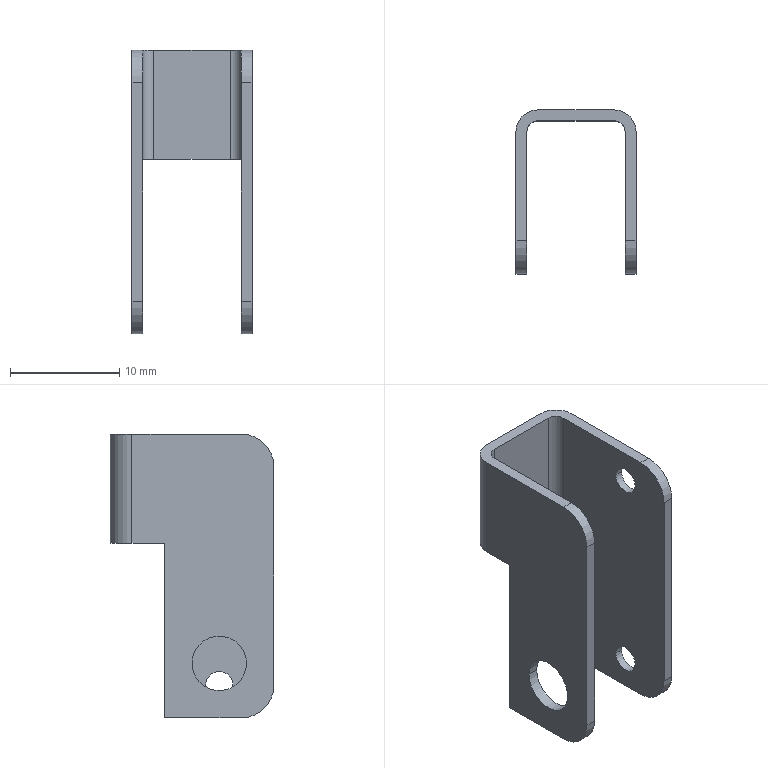Part | NX | 1 solid | 32 faces | box 11 x 15 x 26 mm | volume 658.917 mm3 | plane 14 | cylinder 14 | cone 4 | commonest cylinder face diameters 2.5 x4 6 x4 2 x2 4 x2 5 x2
STEP:
#1=CARTESIAN_POINT('',(0.,10.,0.));
#2=VERTEX_POINT('',#1);
#3=CARTESIAN_POINT('',(1.,10.,0.));
#4=VERTEX_POINT('',#3);
#5=CARTESIAN_POINT('',(0.,10.,0.));
#6=DIRECTION('',(1.,0.,0.));
#7=VECTOR('',#6,1000.);
#8=LINE('',#5,#7);
#9=EDGE_CURVE('',#2,#4,#8,.T.);
#10=ORIENTED_EDGE('',*,*,#9,.T.);
#11=CARTESIAN_POINT('',(1.,3.,0.));
#12=VERTEX_POINT('',#11);
#13=CARTESIAN_POINT('',(1.,0.,0.));
#14=DIRECTION('',(0.,-1.,0.));
#15=VECTOR('',#14,1000.);
#16=LINE('',#13,#15);
#17=EDGE_CURVE('',#4,#12,#16,.T.);
#18=ORIENTED_EDGE('',*,*,#17,.T.);
#19=CARTESIAN_POINT('',(0.,3.,0.));
#20=VERTEX_POINT('',#19);
#21=CARTESIAN_POINT('',(11.047,3.,0.));
#22=DIRECTION('',(-1.,0.,0.));
#23=VECTOR('',#22,1000.);
#24=LINE('',#21,#23);
#25=EDGE_CURVE('',#12,#20,#24,.T.);
#26=ORIENTED_EDGE('',*,*,#25,.T.);
#27=CARTESIAN_POINT('',(0.,0.,0.));
#28=DIRECTION('',(0.,-1.,0.));
#29=VECTOR('',#28,1000.);
#30=LINE('',#27,#29);
#31=EDGE_CURVE('',#2,#20,#30,.T.);
#32=ORIENTED_EDGE('',*,*,#31,.F.);
#33=EDGE_LOOP('',(#10,#18,#26,#32));
#34=FACE_BOUND('',#33,.T.);
#35=CARTESIAN_POINT('',(0.,0.,0.));
#36=DIRECTION('',(0.,0.,1.));
#37=DIRECTION('',(1.,0.,0.));
#38=AXIS2_PLACEMENT_3D('',#35,#36,#37);
#39=PLANE('',#38);
#40=ADVANCED_FACE('',(#34),#39,.F.);
#41=CARTESIAN_POINT('',(1.,10.,16.));
#42=VERTEX_POINT('',#41);
#43=CARTESIAN_POINT('',(0.,10.,16.));
#44=VERTEX_POINT('',#43);
#45=CARTESIAN_POINT('',(0.,10.,16.));
#46=DIRECTION('',(-1.,0.,0.));
#47=VECTOR('',#46,1000.);
#48=LINE('',#45,#47);
#49=EDGE_CURVE('',#42,#44,#48,.T.);
#50=ORIENTED_EDGE('',*,*,#49,.F.);
#51=CARTESIAN_POINT('',(1.,10.,0.));
#52=DIRECTION('',(0.,0.,1.));
#53=VECTOR('',#52,1000.);
#54=LINE('',#51,#53);
#55=EDGE_CURVE('',#4,#42,#54,.T.);
#56=ORIENTED_EDGE('',*,*,#55,.F.);
#57=ORIENTED_EDGE('',*,*,#9,.F.);
#58=CARTESIAN_POINT('',(0.,10.,0.));
#59=DIRECTION('',(0.,0.,1.));
#60=VECTOR('',#59,1000.);
#61=LINE('',#58,#60);
#62=EDGE_CURVE('',#2,#44,#61,.T.);
#63=ORIENTED_EDGE('',*,*,#62,.T.);
#64=EDGE_LOOP('',(#50,#56,#57,#63));
#65=FACE_BOUND('',#64,.T.);
#66=CARTESIAN_POINT('',(11.,10.,16.));
#67=DIRECTION('',(0.,-1.,0.));
#68=DIRECTION('',(0.,0.,-1.));
#69=AXIS2_PLACEMENT_3D('',#66,#67,#68);
#70=PLANE('',#69);
#71=ADVANCED_FACE('',(#65),#70,.F.);
#72=CARTESIAN_POINT('',(10.74,3.75,3.));
#73=VERTEX_POINT('',#72);
#74=CARTESIAN_POINT('',(10.74,6.25,3.));
#75=VERTEX_POINT('',#74);
#76=CARTESIAN_POINT('',(10.74,5.,3.));
#77=DIRECTION('',(1.,0.,0.));
#78=DIRECTION('',(0.,-1.,0.));
#79=AXIS2_PLACEMENT_3D('',#76,#77,#78);
#80=CIRCLE('',#79,1.25);
#81=EDGE_CURVE('',#73,#75,#80,.T.);
#82=ORIENTED_EDGE('',*,*,#81,.T.);
#83=CARTESIAN_POINT('',(10.,6.25,3.));
#84=VERTEX_POINT('',#83);
#85=CARTESIAN_POINT('',(11.,6.25,3.));
#86=DIRECTION('',(1.,0.,0.));
#87=VECTOR('',#86,1000.);
#88=LINE('',#85,#87);
#89=EDGE_CURVE('',#75,#84,#88,.F.);
#90=ORIENTED_EDGE('',*,*,#89,.T.);
#91=CARTESIAN_POINT('',(10.,3.75,3.));
#92=VERTEX_POINT('',#91);
#93=CARTESIAN_POINT('',(10.,5.,3.));
#94=DIRECTION('',(1.,0.,0.));
#95=DIRECTION('',(0.,-1.,0.));
#96=AXIS2_PLACEMENT_3D('',#93,#94,#95);
#97=CIRCLE('',#96,1.25);
#98=EDGE_CURVE('',#92,#84,#97,.T.);
#99=ORIENTED_EDGE('',*,*,#98,.F.);
#100=CARTESIAN_POINT('',(11.,3.75,3.));
#101=DIRECTION('',(1.,0.,0.));
#102=VECTOR('',#101,1000.);
#103=LINE('',#100,#102);
#104=EDGE_CURVE('',#73,#92,#103,.F.);
#105=ORIENTED_EDGE('',*,*,#104,.F.);
#106=EDGE_LOOP('',(#82,#90,#99,#105));
#107=FACE_BOUND('',#106,.T.);
#108=CARTESIAN_POINT('',(11.,5.,3.));
#109=DIRECTION('',(1.,0.,0.));
#110=DIRECTION('',(0.,-1.,0.));
#111=AXIS2_PLACEMENT_3D('',#108,#109,#110);
#112=CYLINDRICAL_SURFACE('',#111,1.25);
#113=ADVANCED_FACE('',(#107),#112,.F.);
#114=ORIENTED_EDGE('',*,*,#62,.F.);
#115=ORIENTED_EDGE('',*,*,#31,.T.);
#116=CARTESIAN_POINT('',(0.,0.,3.));
#117=VERTEX_POINT('',#116);
#118=CARTESIAN_POINT('',(0.,3.,3.));
#119=DIRECTION('',(-1.,0.,0.));
#120=DIRECTION('',(0.,0.,-1.));
#121=AXIS2_PLACEMENT_3D('',#118,#119,#120);
#122=CIRCLE('',#121,3.);
#123=EDGE_CURVE('',#20,#117,#122,.T.);
#124=ORIENTED_EDGE('',*,*,#123,.T.);
#125=CARTESIAN_POINT('',(0.,0.,23.));
#126=VERTEX_POINT('',#125);
#127=CARTESIAN_POINT('',(0.,0.,0.));
#128=DIRECTION('',(0.,0.,-1.));
#129=VECTOR('',#128,1000.);
#130=LINE('',#127,#129);
#131=EDGE_CURVE('',#126,#117,#130,.T.);
#132=ORIENTED_EDGE('',*,*,#131,.F.);
#133=CARTESIAN_POINT('',(0.,3.,26.));
#134=VERTEX_POINT('',#133);
#135=CARTESIAN_POINT('',(0.,3.,23.));
#136=DIRECTION('',(1.,0.,0.));
#137=DIRECTION('',(0.,0.,1.));
#138=AXIS2_PLACEMENT_3D('',#135,#136,#137);
#139=CIRCLE('',#138,3.);
#140=EDGE_CURVE('',#134,#126,#139,.T.);
#141=ORIENTED_EDGE('',*,*,#140,.F.);
#142=CARTESIAN_POINT('',(0.,13.,26.));
#143=VERTEX_POINT('',#142);
#144=CARTESIAN_POINT('',(0.,0.,26.));
#145=DIRECTION('',(0.,-1.,0.));
#146=VECTOR('',#145,1000.);
#147=LINE('',#144,#146);
#148=EDGE_CURVE('',#143,#134,#147,.T.);
#149=ORIENTED_EDGE('',*,*,#148,.F.);
#150=CARTESIAN_POINT('',(0.,13.,16.));
#151=VERTEX_POINT('',#150);
#152=CARTESIAN_POINT('',(0.,13.,26.05));
#153=DIRECTION('',(0.,0.,-1.));
#154=VECTOR('',#153,1000.);
#155=LINE('',#152,#154);
#156=EDGE_CURVE('',#143,#151,#155,.T.);
#157=ORIENTED_EDGE('',*,*,#156,.T.);
#158=CARTESIAN_POINT('',(0.,0.,16.));
#159=DIRECTION('',(0.,1.,0.));
#160=VECTOR('',#159,1000.);
#161=LINE('',#158,#160);
#162=EDGE_CURVE('',#44,#151,#161,.T.);
#163=ORIENTED_EDGE('',*,*,#162,.F.);
#164=EDGE_LOOP('',(#114,#115,#124,#132,#141,#149,#157,#163));
#165=FACE_BOUND('',#164,.T.);
#166=CARTESIAN_POINT('',(0.,2.5,5.));
#167=VERTEX_POINT('',#166);
#168=CARTESIAN_POINT('',(0.,7.5,5.));
#169=VERTEX_POINT('',#168);
#170=CARTESIAN_POINT('',(0.,5.,5.));
#171=DIRECTION('',(1.,0.,0.));
#172=DIRECTION('',(0.,1.,0.));
#173=AXIS2_PLACEMENT_3D('',#170,#171,#172);
#174=CIRCLE('',#173,2.5);
#175=EDGE_CURVE('',#167,#169,#174,.T.);
#176=ORIENTED_EDGE('',*,*,#175,.T.);
#177=CARTESIAN_POINT('',(0.,5.,5.));
#178=DIRECTION('',(1.,0.,0.));
#179=DIRECTION('',(0.,1.,0.));
#180=AXIS2_PLACEMENT_3D('',#177,#178,#179);
#181=CIRCLE('',#180,2.5);
#182=EDGE_CURVE('',#169,#167,#181,.T.);
#183=ORIENTED_EDGE('',*,*,#182,.T.);
#184=EDGE_LOOP('',(#176,#183));
#185=FACE_BOUND('',#184,.T.);
#186=CARTESIAN_POINT('',(0.,15.,0.));
#187=DIRECTION('',(-1.,0.,0.));
#188=DIRECTION('',(0.,0.,1.));
#189=AXIS2_PLACEMENT_3D('',#186,#187,#188);
#190=PLANE('',#189);
#191=ADVANCED_FACE('',(#165,#185),#190,.T.);
#192=ORIENTED_EDGE('',*,*,#49,.T.);
#193=ORIENTED_EDGE('',*,*,#162,.T.);
#194=CARTESIAN_POINT('',(2.,15.,16.));
#195=VERTEX_POINT('',#194);
#196=CARTESIAN_POINT('',(2.,13.,16.));
#197=DIRECTION('',(0.,0.,-1.));
#198=DIRECTION('',(-1.,0.,0.));
#199=AXIS2_PLACEMENT_3D('',#196,#197,#198);
#200=CIRCLE('',#199,2.);
#201=EDGE_CURVE('',#151,#195,#200,.T.);
#202=ORIENTED_EDGE('',*,*,#201,.T.);
#203=CARTESIAN_POINT('',(9.,15.,16.));
#204=VERTEX_POINT('',#203);
#205=CARTESIAN_POINT('',(0.,15.,16.));
#206=DIRECTION('',(1.,0.,0.));
#207=VECTOR('',#206,1000.);
#208=LINE('',#205,#207);
#209=EDGE_CURVE('',#195,#204,#208,.T.);
#210=ORIENTED_EDGE('',*,*,#209,.T.);
#211=CARTESIAN_POINT('',(11.,13.,16.));
#212=VERTEX_POINT('',#211);
#213=CARTESIAN_POINT('',(9.,13.,16.));
#214=DIRECTION('',(0.,0.,-1.));
#215=DIRECTION('',(0.,1.,0.));
#216=AXIS2_PLACEMENT_3D('',#213,#214,#215);
#217=CIRCLE('',#216,2.);
#218=EDGE_CURVE('',#204,#212,#217,.T.);
#219=ORIENTED_EDGE('',*,*,#218,.T.);
#220=CARTESIAN_POINT('',(11.,10.,16.));
#221=VERTEX_POINT('',#220);
#222=CARTESIAN_POINT('',(11.,0.,16.));
#223=DIRECTION('',(0.,-1.,0.));
#224=VECTOR('',#223,1000.);
#225=LINE('',#222,#224);
#226=EDGE_CURVE('',#212,#221,#225,.T.);
#227=ORIENTED_EDGE('',*,*,#226,.T.);
#228=CARTESIAN_POINT('',(10.,10.,16.));
#229=VERTEX_POINT('',#228);
#230=CARTESIAN_POINT('',(0.,10.,16.));
#231=DIRECTION('',(-1.,0.,0.));
#232=VECTOR('',#231,1000.);
#233=LINE('',#230,#232);
#234=EDGE_CURVE('',#221,#229,#233,.T.);
#235=ORIENTED_EDGE('',*,*,#234,.T.);
#236=CARTESIAN_POINT('',(10.,13.,16.));
#237=VERTEX_POINT('',#236);
#238=CARTESIAN_POINT('',(10.,0.,16.));
#239=DIRECTION('',(0.,-1.,0.));
#240=VECTOR('',#239,1000.);
#241=LINE('',#238,#240);
#242=EDGE_CURVE('',#237,#229,#241,.T.);
#243=ORIENTED_EDGE('',*,*,#242,.F.);
#244=CARTESIAN_POINT('',(9.,14.,16.));
#245=VERTEX_POINT('',#244);
#246=CARTESIAN_POINT('',(9.,13.,16.));
#247=DIRECTION('',(0.,0.,-1.));
#248=DIRECTION('',(0.,1.,0.));
#249=AXIS2_PLACEMENT_3D('',#246,#247,#248);
#250=CIRCLE('',#249,1.);
#251=EDGE_CURVE('',#245,#237,#250,.T.);
#252=ORIENTED_EDGE('',*,*,#251,.F.);
#253=CARTESIAN_POINT('',(2.,14.,16.));
#254=VERTEX_POINT('',#253);
#255=CARTESIAN_POINT('',(0.,14.,16.));
#256=DIRECTION('',(1.,0.,0.));
#257=VECTOR('',#256,1000.);
#258=LINE('',#255,#257);
#259=EDGE_CURVE('',#254,#245,#258,.T.);
#260=ORIENTED_EDGE('',*,*,#259,.F.);
#261=CARTESIAN_POINT('',(1.,13.,16.));
#262=VERTEX_POINT('',#261);
#263=CARTESIAN_POINT('',(2.,13.,16.));
#264=DIRECTION('',(0.,0.,-1.));
#265=DIRECTION('',(-1.,0.,0.));
#266=AXIS2_PLACEMENT_3D('',#263,#264,#265);
#267=CIRCLE('',#266,1.);
#268=EDGE_CURVE('',#262,#254,#267,.T.);
#269=ORIENTED_EDGE('',*,*,#268,.F.);
#270=CARTESIAN_POINT('',(1.,0.,16.));
#271=DIRECTION('',(0.,1.,0.));
#272=VECTOR('',#271,1000.);
#273=LINE('',#270,#272);
#274=EDGE_CURVE('',#42,#262,#273,.T.);
#275=ORIENTED_EDGE('',*,*,#274,.F.);
#276=EDGE_LOOP('',(#192,#193,#202,#210,#219,#227,#235,#243,#252,#260,#269,#275));
#277=FACE_BOUND('',#276,.T.);
#278=CARTESIAN_POINT('',(11.,15.,16.));
#279=DIRECTION('',(0.,0.,1.));
#280=DIRECTION('',(1.,0.,0.));
#281=AXIS2_PLACEMENT_3D('',#278,#279,#280);
#282=PLANE('',#281);
#283=ADVANCED_FACE('',(#277),#282,.F.);
#284=ORIENTED_EDGE('',*,*,#268,.T.);
#285=CARTESIAN_POINT('',(2.,14.,26.));
#286=VERTEX_POINT('',#285);
#287=CARTESIAN_POINT('',(2.,14.,26.));
#288=DIRECTION('',(0.,0.,-1.));
#289=VECTOR('',#288,1000.);
#290=LINE('',#287,#289);
#291=EDGE_CURVE('',#286,#254,#290,.T.);
#292=ORIENTED_EDGE('',*,*,#291,.F.);
#293=CARTESIAN_POINT('',(1.,13.,26.));
#294=VERTEX_POINT('',#293);
#295=CARTESIAN_POINT('',(2.,13.,26.));
#296=DIRECTION('',(0.,0.,1.));
#297=DIRECTION('',(0.,1.,0.));
#298=AXIS2_PLACEMENT_3D('',#295,#296,#297);
#299=CIRCLE('',#298,1.);
#300=EDGE_CURVE('',#286,#294,#299,.T.);
#301=ORIENTED_EDGE('',*,*,#300,.T.);
#302=CARTESIAN_POINT('',(1.,13.,26.05));
#303=DIRECTION('',(0.,0.,-1.));
#304=VECTOR('',#303,1000.);
#305=LINE('',#302,#304);
#306=EDGE_CURVE('',#294,#262,#305,.T.);
#307=ORIENTED_EDGE('',*,*,#306,.T.);
#308=EDGE_LOOP('',(#284,#292,#301,#307));
#309=FACE_BOUND('',#308,.T.);
#310=CARTESIAN_POINT('',(2.,13.,26.05));
#311=DIRECTION('',(0.,0.,-1.));
#312=DIRECTION('',(-1.,0.,0.));
#313=AXIS2_PLACEMENT_3D('',#310,#311,#312);
#314=CYLINDRICAL_SURFACE('',#313,1.);
#315=ADVANCED_FACE('',(#309),#314,.F.);
#316=CARTESIAN_POINT('',(10.,3.,26.));
#317=VERTEX_POINT('',#316);
#318=CARTESIAN_POINT('',(11.,3.,26.));
#319=VERTEX_POINT('',#318);
#320=CARTESIAN_POINT('',(-0.04916,3.,26.));
#321=DIRECTION('',(1.,0.,0.));
#322=VECTOR('',#321,1000.);
#323=LINE('',#320,#322);
#324=EDGE_CURVE('',#317,#319,#323,.T.);
#325=ORIENTED_EDGE('',*,*,#324,.T.);
#326=CARTESIAN_POINT('',(11.,13.,26.));
#327=VERTEX_POINT('',#326);
#328=CARTESIAN_POINT('',(11.,0.,26.));
#329=DIRECTION('',(0.,1.,0.));
#330=VECTOR('',#329,1000.);
#331=LINE('',#328,#330);
#332=EDGE_CURVE('',#319,#327,#331,.T.);
#333=ORIENTED_EDGE('',*,*,#332,.T.);
#334=CARTESIAN_POINT('',(9.,15.,26.));
#335=VERTEX_POINT('',#334);
#336=CARTESIAN_POINT('',(9.,13.,26.));
#337=DIRECTION('',(0.,0.,-1.));
#338=DIRECTION('',(0.,1.,0.));
#339=AXIS2_PLACEMENT_3D('',#336,#337,#338);
#340=CIRCLE('',#339,2.);
#341=EDGE_CURVE('',#335,#327,#340,.T.);
#342=ORIENTED_EDGE('',*,*,#341,.F.);
#343=CARTESIAN_POINT('',(2.,15.,26.));
#344=VERTEX_POINT('',#343);
#345=CARTESIAN_POINT('',(2.,15.,26.));
#346=DIRECTION('',(1.,0.,0.));
#347=VECTOR('',#346,1000.);
#348=LINE('',#345,#347);
#349=EDGE_CURVE('',#344,#335,#348,.T.);
#350=ORIENTED_EDGE('',*,*,#349,.F.);
#351=CARTESIAN_POINT('',(2.,13.,26.));
#352=DIRECTION('',(0.,0.,-1.));
#353=DIRECTION('',(-1.,0.,0.));
#354=AXIS2_PLACEMENT_3D('',#351,#352,#353);
#355=CIRCLE('',#354,2.);
#356=EDGE_CURVE('',#143,#344,#355,.T.);
#357=ORIENTED_EDGE('',*,*,#356,.F.);
#358=ORIENTED_EDGE('',*,*,#148,.T.);
#359=CARTESIAN_POINT('',(1.,3.,26.));
#360=VERTEX_POINT('',#359);
#361=CARTESIAN_POINT('',(-0.04916,3.,26.));
#362=DIRECTION('',(1.,0.,0.));
#363=VECTOR('',#362,1000.);
#364=LINE('',#361,#363);
#365=EDGE_CURVE('',#134,#360,#364,.T.);
#366=ORIENTED_EDGE('',*,*,#365,.T.);
#367=CARTESIAN_POINT('',(1.,0.,26.));
#368=DIRECTION('',(0.,-1.,0.));
#369=VECTOR('',#368,1000.);
#370=LINE('',#367,#369);
#371=EDGE_CURVE('',#294,#360,#370,.T.);
#372=ORIENTED_EDGE('',*,*,#371,.F.);
#373=ORIENTED_EDGE('',*,*,#300,.F.);
#374=CARTESIAN_POINT('',(9.,14.,26.));
#375=VERTEX_POINT('',#374);
#376=CARTESIAN_POINT('',(2.,14.,26.));
#377=DIRECTION('',(1.,0.,0.));
#378=VECTOR('',#377,1000.);
#379=LINE('',#376,#378);
#380=EDGE_CURVE('',#286,#375,#379,.T.);
#381=ORIENTED_EDGE('',*,*,#380,.T.);
#382=CARTESIAN_POINT('',(10.,13.,26.));
#383=VERTEX_POINT('',#382);
#384=CARTESIAN_POINT('',(9.,13.,26.));
#385=DIRECTION('',(0.,0.,1.));
#386=DIRECTION('',(1.,0.,0.));
#387=AXIS2_PLACEMENT_3D('',#384,#385,#386);
#388=CIRCLE('',#387,1.);
#389=EDGE_CURVE('',#383,#375,#388,.T.);
#390=ORIENTED_EDGE('',*,*,#389,.F.);
#391=CARTESIAN_POINT('',(10.,0.,26.));
#392=DIRECTION('',(0.,1.,0.));
#393=VECTOR('',#392,1000.);
#394=LINE('',#391,#393);
#395=EDGE_CURVE('',#317,#383,#394,.T.);
#396=ORIENTED_EDGE('',*,*,#395,.F.);
#397=EDGE_LOOP('',(#325,#333,#342,#350,#357,#358,#366,#372,#373,#381,#390,#396));
#398=FACE_BOUND('',#397,.T.);
#399=CARTESIAN_POINT('',(0.,0.,26.));
#400=DIRECTION('',(0.,0.,1.));
#401=DIRECTION('',(1.,0.,0.));
#402=AXIS2_PLACEMENT_3D('',#399,#400,#401);
#403=PLANE('',#402);
#404=ADVANCED_FACE('',(#398),#403,.T.);
#405=CARTESIAN_POINT('',(11.,0.,23.));
#406=VERTEX_POINT('',#405);
#407=CARTESIAN_POINT('',(10.,0.,23.));
#408=VERTEX_POINT('',#407);
#409=CARTESIAN_POINT('',(11.,0.,23.));
#410=DIRECTION('',(-1.,0.,0.));
#411=VECTOR('',#410,1000.);
#412=LINE('',#409,#411);
#413=EDGE_CURVE('',#406,#408,#412,.T.);
#414=ORIENTED_EDGE('',*,*,#413,.F.);
#415=CARTESIAN_POINT('',(11.,3.,23.));
#416=DIRECTION('',(1.,0.,0.));
#417=DIRECTION('',(0.,0.,1.));
#418=AXIS2_PLACEMENT_3D('',#415,#416,#417);
#419=CIRCLE('',#418,3.);
#420=EDGE_CURVE('',#319,#406,#419,.T.);
#421=ORIENTED_EDGE('',*,*,#420,.F.);
#422=ORIENTED_EDGE('',*,*,#324,.F.);
#423=CARTESIAN_POINT('',(10.,3.,23.));
#424=DIRECTION('',(1.,0.,0.));
#425=DIRECTION('',(0.,0.,1.));
#426=AXIS2_PLACEMENT_3D('',#423,#424,#425);
#427=CIRCLE('',#426,3.);
#428=EDGE_CURVE('',#317,#408,#427,.T.);
#429=ORIENTED_EDGE('',*,*,#428,.T.);
#430=EDGE_LOOP('',(#414,#421,#422,#429));
#431=FACE_BOUND('',#430,.T.);
#432=CARTESIAN_POINT('',(-0.04916,3.,23.));
#433=DIRECTION('',(1.,0.,0.));
#434=DIRECTION('',(0.,0.,1.));
#435=AXIS2_PLACEMENT_3D('',#432,#433,#434);
#436=CYLINDRICAL_SURFACE('',#435,3.);
#437=ADVANCED_FACE('',(#431),#436,.T.);
#438=ORIENTED_EDGE('',*,*,#413,.T.);
#439=CARTESIAN_POINT('',(10.,0.,3.));
#440=VERTEX_POINT('',#439);
#441=CARTESIAN_POINT('',(10.,0.,0.));
#442=DIRECTION('',(0.,0.,1.));
#443=VECTOR('',#442,1000.);
#444=LINE('',#441,#443);
#445=EDGE_CURVE('',#440,#408,#444,.T.);
#446=ORIENTED_EDGE('',*,*,#445,.F.);
#447=CARTESIAN_POINT('',(11.,0.,3.));
#448=VERTEX_POINT('',#447);
#449=CARTESIAN_POINT('',(10.,0.,3.));
#450=DIRECTION('',(1.,0.,0.));
#451=VECTOR('',#450,1000.);
#452=LINE('',#449,#451);
#453=EDGE_CURVE('',#440,#448,#452,.T.);
#454=ORIENTED_EDGE('',*,*,#453,.T.);
#455=CARTESIAN_POINT('',(11.,0.,0.));
#456=DIRECTION('',(0.,0.,1.));
#457=VECTOR('',#456,1000.);
#458=LINE('',#455,#457);
#459=EDGE_CURVE('',#448,#406,#458,.T.);
#460=ORIENTED_EDGE('',*,*,#459,.T.);
#461=EDGE_LOOP('',(#438,#446,#454,#460));
#462=FACE_BOUND('',#461,.T.);
#463=CARTESIAN_POINT('',(0.,0.,0.));
#464=DIRECTION('',(0.,-1.,0.));
#465=DIRECTION('',(0.,0.,-1.));
#466=AXIS2_PLACEMENT_3D('',#463,#464,#465);
#467=PLANE('',#466);
#468=ADVANCED_FACE('',(#462),#467,.T.);
#469=ORIENTED_EDGE('',*,*,#226,.F.);
#470=CARTESIAN_POINT('',(11.,13.,16.));
#471=DIRECTION('',(0.,0.,1.));
#472=VECTOR('',#471,1000.);
#473=LINE('',#470,#472);
#474=EDGE_CURVE('',#212,#327,#473,.T.);
#475=ORIENTED_EDGE('',*,*,#474,.T.);
#476=ORIENTED_EDGE('',*,*,#332,.F.);
#477=ORIENTED_EDGE('',*,*,#420,.T.);
#478=ORIENTED_EDGE('',*,*,#459,.F.);
#479=CARTESIAN_POINT('',(11.,3.,0.));
#480=VERTEX_POINT('',#479);
#481=CARTESIAN_POINT('',(11.,3.,3.));
#482=DIRECTION('',(-1.,0.,0.));
#483=DIRECTION('',(0.,0.,-1.));
#484=AXIS2_PLACEMENT_3D('',#481,#482,#483);
#485=CIRCLE('',#484,3.);
#486=EDGE_CURVE('',#480,#448,#485,.T.);
#487=ORIENTED_EDGE('',*,*,#486,.F.);
#488=CARTESIAN_POINT('',(11.,10.,0.));
#489=VERTEX_POINT('',#488);
#490=CARTESIAN_POINT('',(11.,0.,0.));
#491=DIRECTION('',(0.,1.,0.));
#492=VECTOR('',#491,1000.);
#493=LINE('',#490,#492);
#494=EDGE_CURVE('',#480,#489,#493,.T.);
#495=ORIENTED_EDGE('',*,*,#494,.T.);
#496=CARTESIAN_POINT('',(11.,10.,0.));
#497=DIRECTION('',(0.,0.,1.));
#498=VECTOR('',#497,1000.);
#499=LINE('',#496,#498);
#500=EDGE_CURVE('',#489,#221,#499,.T.);
#501=ORIENTED_EDGE('',*,*,#500,.T.);
#502=EDGE_LOOP('',(#469,#475,#476,#477,#478,#487,#495,#501));
#503=FACE_BOUND('',#502,.T.);
#504=CARTESIAN_POINT('',(11.,3.3,23.));
#505=VERTEX_POINT('',#504);
#506=CARTESIAN_POINT('',(11.,6.7,23.));
#507=VERTEX_POINT('',#506);
#508=CARTESIAN_POINT('',(11.,5.,23.));
#509=DIRECTION('',(1.,0.,0.));
#510=DIRECTION('',(0.,-1.,0.));
#511=AXIS2_PLACEMENT_3D('',#508,#509,#510);
#512=CIRCLE('',#511,1.7);
#513=EDGE_CURVE('',#505,#507,#512,.T.);
#514=ORIENTED_EDGE('',*,*,#513,.F.);
#515=CARTESIAN_POINT('',(11.,5.,23.));
#516=DIRECTION('',(1.,0.,0.));
#517=DIRECTION('',(0.,-1.,0.));
#518=AXIS2_PLACEMENT_3D('',#515,#516,#517);
#519=CIRCLE('',#518,1.7);
#520=EDGE_CURVE('',#507,#505,#519,.T.);
#521=ORIENTED_EDGE('',*,*,#520,.F.);
#522=EDGE_LOOP('',(#514,#521));
#523=FACE_BOUND('',#522,.T.);
#524=CARTESIAN_POINT('',(11.,3.3,3.));
#525=VERTEX_POINT('',#524);
#526=CARTESIAN_POINT('',(11.,6.7,3.));
#527=VERTEX_POINT('',#526);
#528=CARTESIAN_POINT('',(11.,5.,3.));
#529=DIRECTION('',(1.,0.,0.));
#530=DIRECTION('',(0.,-1.,0.));
#531=AXIS2_PLACEMENT_3D('',#528,#529,#530);
#532=CIRCLE('',#531,1.7);
#533=EDGE_CURVE('',#525,#527,#532,.T.);
#534=ORIENTED_EDGE('',*,*,#533,.F.);
#535=CARTESIAN_POINT('',(11.,5.,3.));
#536=DIRECTION('',(1.,0.,0.));
#537=DIRECTION('',(0.,-1.,0.));
#538=AXIS2_PLACEMENT_3D('',#535,#536,#537);
#539=CIRCLE('',#538,1.7);
#540=EDGE_CURVE('',#527,#525,#539,.T.);
#541=ORIENTED_EDGE('',*,*,#540,.F.);
#542=EDGE_LOOP('',(#534,#541));
#543=FACE_BOUND('',#542,.T.);
#544=CARTESIAN_POINT('',(11.,0.,0.));
#545=DIRECTION('',(1.,0.,0.));
#546=DIRECTION('',(0.,1.,0.));
#547=AXIS2_PLACEMENT_3D('',#544,#545,#546);
#548=PLANE('',#547);
#549=ADVANCED_FACE('',(#503,#523,#543),#548,.T.);
#550=ORIENTED_EDGE('',*,*,#533,.T.);
#551=CARTESIAN_POINT('',(10.74,6.25,3.));
#552=DIRECTION('',(0.5,0.866,0.));
#553=VECTOR('',#552,1000.);
#554=LINE('',#551,#553);
#555=EDGE_CURVE('',#527,#75,#554,.F.);
#556=ORIENTED_EDGE('',*,*,#555,.T.);
#557=ORIENTED_EDGE('',*,*,#81,.F.);
#558=CARTESIAN_POINT('',(10.74,3.75,3.));
#559=DIRECTION('',(0.5,-0.866,0.));
#560=VECTOR('',#559,1000.);
#561=LINE('',#558,#560);
#562=EDGE_CURVE('',#525,#73,#561,.F.);
#563=ORIENTED_EDGE('',*,*,#562,.F.);
#564=EDGE_LOOP('',(#550,#556,#557,#563));
#565=FACE_BOUND('',#564,.T.);
#566=CARTESIAN_POINT('',(10.74,5.,3.));
#567=DIRECTION('',(1.,0.,0.));
#568=DIRECTION('',(0.,-1.,0.));
#569=AXIS2_PLACEMENT_3D('',#566,#567,#568);
#570=CONICAL_SURFACE('',#569,1.25,1.047);
#571=ADVANCED_FACE('',(#565),#570,.F.);
#572=ORIENTED_EDGE('',*,*,#234,.F.);
#573=ORIENTED_EDGE('',*,*,#500,.F.);
#574=CARTESIAN_POINT('',(10.,10.,0.));
#575=VERTEX_POINT('',#574);
#576=CARTESIAN_POINT('',(0.,10.,0.));
#577=DIRECTION('',(1.,0.,0.));
#578=VECTOR('',#577,1000.);
#579=LINE('',#576,#578);
#580=EDGE_CURVE('',#575,#489,#579,.T.);
#581=ORIENTED_EDGE('',*,*,#580,.F.);
#582=CARTESIAN_POINT('',(10.,10.,0.));
#583=DIRECTION('',(0.,0.,-1.));
#584=VECTOR('',#583,1000.);
#585=LINE('',#582,#584);
#586=EDGE_CURVE('',#229,#575,#585,.T.);
#587=ORIENTED_EDGE('',*,*,#586,.F.);
#588=EDGE_LOOP('',(#572,#573,#581,#587));
#589=FACE_BOUND('',#588,.T.);
#590=CARTESIAN_POINT('',(11.,10.,16.));
#591=DIRECTION('',(0.,-1.,0.));
#592=DIRECTION('',(0.,0.,-1.));
#593=AXIS2_PLACEMENT_3D('',#590,#591,#592);
#594=PLANE('',#593);
#595=ADVANCED_FACE('',(#589),#594,.F.);
#596=ORIENTED_EDGE('',*,*,#586,.T.);
#597=CARTESIAN_POINT('',(10.,3.,0.));
#598=VERTEX_POINT('',#597);
#599=CARTESIAN_POINT('',(10.,0.,0.));
#600=DIRECTION('',(0.,1.,0.));
#601=VECTOR('',#600,1000.);
#602=LINE('',#599,#601);
#603=EDGE_CURVE('',#598,#575,#602,.T.);
#604=ORIENTED_EDGE('',*,*,#603,.F.);
#605=CARTESIAN_POINT('',(10.,3.,3.));
#606=DIRECTION('',(-1.,0.,0.));
#607=DIRECTION('',(0.,0.,-1.));
#608=AXIS2_PLACEMENT_3D('',#605,#606,#607);
#609=CIRCLE('',#608,3.);
#610=EDGE_CURVE('',#598,#440,#609,.T.);
#611=ORIENTED_EDGE('',*,*,#610,.T.);
#612=ORIENTED_EDGE('',*,*,#445,.T.);
#613=ORIENTED_EDGE('',*,*,#428,.F.);
#614=ORIENTED_EDGE('',*,*,#395,.T.);
#615=CARTESIAN_POINT('',(10.,13.,26.));
#616=DIRECTION('',(0.,0.,-1.));
#617=VECTOR('',#616,1000.);
#618=LINE('',#615,#617);
#619=EDGE_CURVE('',#383,#237,#618,.T.);
#620=ORIENTED_EDGE('',*,*,#619,.T.);
#621=ORIENTED_EDGE('',*,*,#242,.T.);
#622=EDGE_LOOP('',(#596,#604,#611,#612,#613,#614,#620,#621));
#623=FACE_BOUND('',#622,.T.);
#624=CARTESIAN_POINT('',(10.,6.25,23.));
#625=VERTEX_POINT('',#624);
#626=CARTESIAN_POINT('',(10.,3.75,23.));
#627=VERTEX_POINT('',#626);
#628=CARTESIAN_POINT('',(10.,5.,23.));
#629=DIRECTION('',(1.,0.,0.));
#630=DIRECTION('',(0.,-1.,0.));
#631=AXIS2_PLACEMENT_3D('',#628,#629,#630);
#632=CIRCLE('',#631,1.25);
#633=EDGE_CURVE('',#625,#627,#632,.T.);
#634=ORIENTED_EDGE('',*,*,#633,.T.);
#635=CARTESIAN_POINT('',(10.,5.,23.));
#636=DIRECTION('',(1.,0.,0.));
#637=DIRECTION('',(0.,-1.,0.));
#638=AXIS2_PLACEMENT_3D('',#635,#636,#637);
#639=CIRCLE('',#638,1.25);
#640=EDGE_CURVE('',#627,#625,#639,.T.);
#641=ORIENTED_EDGE('',*,*,#640,.T.);
#642=EDGE_LOOP('',(#634,#641));
#643=FACE_BOUND('',#642,.T.);
#644=ORIENTED_EDGE('',*,*,#98,.T.);
#645=CARTESIAN_POINT('',(10.,5.,3.));
#646=DIRECTION('',(1.,0.,0.));
#647=DIRECTION('',(0.,-1.,0.));
#648=AXIS2_PLACEMENT_3D('',#645,#646,#647);
#649=CIRCLE('',#648,1.25);
#650=EDGE_CURVE('',#84,#92,#649,.T.);
#651=ORIENTED_EDGE('',*,*,#650,.T.);
#652=EDGE_LOOP('',(#644,#651));
#653=FACE_BOUND('',#652,.T.);
#654=CARTESIAN_POINT('',(10.,0.,0.));
#655=DIRECTION('',(1.,0.,0.));
#656=DIRECTION('',(0.,1.,0.));
#657=AXIS2_PLACEMENT_3D('',#654,#655,#656);
#658=PLANE('',#657);
#659=ADVANCED_FACE('',(#623,#643,#653),#658,.F.);
#660=ORIENTED_EDGE('',*,*,#251,.T.);
#661=ORIENTED_EDGE('',*,*,#619,.F.);
#662=ORIENTED_EDGE('',*,*,#389,.T.);
#663=CARTESIAN_POINT('',(9.,14.,26.05));
#664=DIRECTION('',(0.,0.,-1.));
#665=VECTOR('',#664,1000.);
#666=LINE('',#663,#665);
#667=EDGE_CURVE('',#375,#245,#666,.T.);
#668=ORIENTED_EDGE('',*,*,#667,.T.);
#669=EDGE_LOOP('',(#660,#661,#662,#668));
#670=FACE_BOUND('',#669,.T.);
#671=CARTESIAN_POINT('',(9.,13.,26.05));
#672=DIRECTION('',(0.,0.,-1.));
#673=DIRECTION('',(0.,1.,0.));
#674=AXIS2_PLACEMENT_3D('',#671,#672,#673);
#675=CYLINDRICAL_SURFACE('',#674,1.);
#676=ADVANCED_FACE('',(#670),#675,.F.);
#677=ORIENTED_EDGE('',*,*,#259,.T.);
#678=ORIENTED_EDGE('',*,*,#667,.F.);
#679=ORIENTED_EDGE('',*,*,#380,.F.);
#680=ORIENTED_EDGE('',*,*,#291,.T.);
#681=EDGE_LOOP('',(#677,#678,#679,#680));
#682=FACE_BOUND('',#681,.T.);
#683=CARTESIAN_POINT('',(11.,14.,0.));
#684=DIRECTION('',(0.,1.,0.));
#685=DIRECTION('',(1.,0.,0.));
#686=AXIS2_PLACEMENT_3D('',#683,#684,#685);
#687=PLANE('',#686);
#688=ADVANCED_FACE('',(#682),#687,.F.);
#689=ORIENTED_EDGE('',*,*,#453,.F.);
#690=ORIENTED_EDGE('',*,*,#610,.F.);
#691=CARTESIAN_POINT('',(11.047,3.,0.));
#692=DIRECTION('',(-1.,0.,0.));
#693=VECTOR('',#692,1000.);
#694=LINE('',#691,#693);
#695=EDGE_CURVE('',#480,#598,#694,.T.);
#696=ORIENTED_EDGE('',*,*,#695,.F.);
#697=ORIENTED_EDGE('',*,*,#486,.T.);
#698=EDGE_LOOP('',(#689,#690,#696,#697));
#699=FACE_BOUND('',#698,.T.);
#700=CARTESIAN_POINT('',(11.047,3.,3.));
#701=DIRECTION('',(-1.,0.,0.));
#702=DIRECTION('',(0.,0.,-1.));
#703=AXIS2_PLACEMENT_3D('',#700,#701,#702);
#704=CYLINDRICAL_SURFACE('',#703,3.);
#705=ADVANCED_FACE('',(#699),#704,.T.);
#706=ORIENTED_EDGE('',*,*,#580,.T.);
#707=ORIENTED_EDGE('',*,*,#494,.F.);
#708=ORIENTED_EDGE('',*,*,#695,.T.);
#709=ORIENTED_EDGE('',*,*,#603,.T.);
#710=EDGE_LOOP('',(#706,#707,#708,#709));
#711=FACE_BOUND('',#710,.T.);
#712=CARTESIAN_POINT('',(0.,0.,0.));
#713=DIRECTION('',(0.,0.,1.));
#714=DIRECTION('',(1.,0.,0.));
#715=AXIS2_PLACEMENT_3D('',#712,#713,#714);
#716=PLANE('',#715);
#717=ADVANCED_FACE('',(#711),#716,.F.);
#718=CARTESIAN_POINT('',(1.,0.,23.));
#719=VERTEX_POINT('',#718);
#720=CARTESIAN_POINT('',(1.,0.,23.));
#721=DIRECTION('',(-1.,0.,0.));
#722=VECTOR('',#721,1000.);
#723=LINE('',#720,#722);
#724=EDGE_CURVE('',#719,#126,#723,.T.);
#725=ORIENTED_EDGE('',*,*,#724,.F.);
#726=CARTESIAN_POINT('',(1.,3.,23.));
#727=DIRECTION('',(1.,0.,0.));
#728=DIRECTION('',(0.,0.,1.));
#729=AXIS2_PLACEMENT_3D('',#726,#727,#728);
#730=CIRCLE('',#729,3.);
#731=EDGE_CURVE('',#360,#719,#730,.T.);
#732=ORIENTED_EDGE('',*,*,#731,.F.);
#733=ORIENTED_EDGE('',*,*,#365,.F.);
#734=ORIENTED_EDGE('',*,*,#140,.T.);
#735=EDGE_LOOP('',(#725,#732,#733,#734));
#736=FACE_BOUND('',#735,.T.);
#737=CARTESIAN_POINT('',(-0.04916,3.,23.));
#738=DIRECTION('',(1.,0.,0.));
#739=DIRECTION('',(0.,0.,1.));
#740=AXIS2_PLACEMENT_3D('',#737,#738,#739);
#741=CYLINDRICAL_SURFACE('',#740,3.);
#742=ADVANCED_FACE('',(#736),#741,.T.);
#743=ORIENTED_EDGE('',*,*,#175,.F.);
#744=CARTESIAN_POINT('',(1.,2.5,5.));
#745=VERTEX_POINT('',#744);
#746=CARTESIAN_POINT('',(0.,2.5,5.));
#747=DIRECTION('',(1.,0.,0.));
#748=VECTOR('',#747,1000.);
#749=LINE('',#746,#748);
#750=EDGE_CURVE('',#167,#745,#749,.T.);
#751=ORIENTED_EDGE('',*,*,#750,.T.);
#752=CARTESIAN_POINT('',(1.,7.5,5.));
#753=VERTEX_POINT('',#752);
#754=CARTESIAN_POINT('',(1.,5.,5.));
#755=DIRECTION('',(1.,0.,0.));
#756=DIRECTION('',(0.,1.,0.));
#757=AXIS2_PLACEMENT_3D('',#754,#755,#756);
#758=CIRCLE('',#757,2.5);
#759=EDGE_CURVE('',#745,#753,#758,.T.);
#760=ORIENTED_EDGE('',*,*,#759,.T.);
#761=CARTESIAN_POINT('',(0.,7.5,5.));
#762=DIRECTION('',(1.,0.,0.));
#763=VECTOR('',#762,1000.);
#764=LINE('',#761,#763);
#765=EDGE_CURVE('',#169,#753,#764,.T.);
#766=ORIENTED_EDGE('',*,*,#765,.F.);
#767=EDGE_LOOP('',(#743,#751,#760,#766));
#768=FACE_BOUND('',#767,.T.);
#769=CARTESIAN_POINT('',(0.,5.,5.));
#770=DIRECTION('',(1.,0.,0.));
#771=DIRECTION('',(0.,1.,0.));
#772=AXIS2_PLACEMENT_3D('',#769,#770,#771);
#773=CYLINDRICAL_SURFACE('',#772,2.5);
#774=ADVANCED_FACE('',(#768),#773,.F.);
#775=ORIENTED_EDGE('',*,*,#724,.T.);
#776=ORIENTED_EDGE('',*,*,#131,.T.);
#777=CARTESIAN_POINT('',(1.,0.,3.));
#778=VERTEX_POINT('',#777);
#779=CARTESIAN_POINT('',(0.,0.,3.));
#780=DIRECTION('',(1.,0.,0.));
#781=VECTOR('',#780,1000.);
#782=LINE('',#779,#781);
#783=EDGE_CURVE('',#117,#778,#782,.T.);
#784=ORIENTED_EDGE('',*,*,#783,.T.);
#785=CARTESIAN_POINT('',(1.,0.,0.));
#786=DIRECTION('',(0.,0.,-1.));
#787=VECTOR('',#786,1000.);
#788=LINE('',#785,#787);
#789=EDGE_CURVE('',#719,#778,#788,.T.);
#790=ORIENTED_EDGE('',*,*,#789,.F.);
#791=EDGE_LOOP('',(#775,#776,#784,#790));
#792=FACE_BOUND('',#791,.T.);
#793=CARTESIAN_POINT('',(0.,0.,0.));
#794=DIRECTION('',(0.,-1.,0.));
#795=DIRECTION('',(0.,0.,-1.));
#796=AXIS2_PLACEMENT_3D('',#793,#794,#795);
#797=PLANE('',#796);
#798=ADVANCED_FACE('',(#792),#797,.T.);
#799=ORIENTED_EDGE('',*,*,#783,.F.);
#800=ORIENTED_EDGE('',*,*,#123,.F.);
#801=ORIENTED_EDGE('',*,*,#25,.F.);
#802=CARTESIAN_POINT('',(1.,3.,3.));
#803=DIRECTION('',(-1.,0.,0.));
#804=DIRECTION('',(0.,0.,-1.));
#805=AXIS2_PLACEMENT_3D('',#802,#803,#804);
#806=CIRCLE('',#805,3.);
#807=EDGE_CURVE('',#12,#778,#806,.T.);
#808=ORIENTED_EDGE('',*,*,#807,.T.);
#809=EDGE_LOOP('',(#799,#800,#801,#808));
#810=FACE_BOUND('',#809,.T.);
#811=CARTESIAN_POINT('',(11.047,3.,3.));
#812=DIRECTION('',(-1.,0.,0.));
#813=DIRECTION('',(0.,0.,-1.));
#814=AXIS2_PLACEMENT_3D('',#811,#812,#813);
#815=CYLINDRICAL_SURFACE('',#814,3.);
#816=ADVANCED_FACE('',(#810),#815,.T.);
#817=ORIENTED_EDGE('',*,*,#218,.F.);
#818=CARTESIAN_POINT('',(9.,15.,26.05));
#819=DIRECTION('',(0.,0.,-1.));
#820=VECTOR('',#819,1000.);
#821=LINE('',#818,#820);
#822=EDGE_CURVE('',#335,#204,#821,.T.);
#823=ORIENTED_EDGE('',*,*,#822,.F.);
#824=ORIENTED_EDGE('',*,*,#341,.T.);
#825=ORIENTED_EDGE('',*,*,#474,.F.);
#826=EDGE_LOOP('',(#817,#823,#824,#825));
#827=FACE_BOUND('',#826,.T.);
#828=CARTESIAN_POINT('',(9.,13.,26.05));
#829=DIRECTION('',(0.,0.,-1.));
#830=DIRECTION('',(0.,1.,0.));
#831=AXIS2_PLACEMENT_3D('',#828,#829,#830);
#832=CYLINDRICAL_SURFACE('',#831,2.);
#833=ADVANCED_FACE('',(#827),#832,.T.);
#834=ORIENTED_EDGE('',*,*,#209,.F.);
#835=CARTESIAN_POINT('',(2.,15.,16.));
#836=DIRECTION('',(0.,0.,1.));
#837=VECTOR('',#836,1000.);
#838=LINE('',#835,#837);
#839=EDGE_CURVE('',#195,#344,#838,.T.);
#840=ORIENTED_EDGE('',*,*,#839,.T.);
#841=ORIENTED_EDGE('',*,*,#349,.T.);
#842=ORIENTED_EDGE('',*,*,#822,.T.);
#843=EDGE_LOOP('',(#834,#840,#841,#842));
#844=FACE_BOUND('',#843,.T.);
#845=CARTESIAN_POINT('',(11.,15.,0.));
#846=DIRECTION('',(0.,1.,0.));
#847=DIRECTION('',(1.,0.,0.));
#848=AXIS2_PLACEMENT_3D('',#845,#846,#847);
#849=PLANE('',#848);
#850=ADVANCED_FACE('',(#844),#849,.T.);
#851=ORIENTED_EDGE('',*,*,#201,.F.);
#852=ORIENTED_EDGE('',*,*,#156,.F.);
#853=ORIENTED_EDGE('',*,*,#356,.T.);
#854=ORIENTED_EDGE('',*,*,#839,.F.);
#855=EDGE_LOOP('',(#851,#852,#853,#854));
#856=FACE_BOUND('',#855,.T.);
#857=CARTESIAN_POINT('',(2.,13.,26.05));
#858=DIRECTION('',(0.,0.,-1.));
#859=DIRECTION('',(-1.,0.,0.));
#860=AXIS2_PLACEMENT_3D('',#857,#858,#859);
#861=CYLINDRICAL_SURFACE('',#860,2.);
#862=ADVANCED_FACE('',(#856),#861,.T.);
#863=ORIENTED_EDGE('',*,*,#274,.T.);
#864=ORIENTED_EDGE('',*,*,#306,.F.);
#865=ORIENTED_EDGE('',*,*,#371,.T.);
#866=ORIENTED_EDGE('',*,*,#731,.T.);
#867=ORIENTED_EDGE('',*,*,#789,.T.);
#868=ORIENTED_EDGE('',*,*,#807,.F.);
#869=ORIENTED_EDGE('',*,*,#17,.F.);
#870=ORIENTED_EDGE('',*,*,#55,.T.);
#871=EDGE_LOOP('',(#863,#864,#865,#866,#867,#868,#869,#870));
#872=FACE_BOUND('',#871,.T.);
#873=ORIENTED_EDGE('',*,*,#759,.F.);
#874=CARTESIAN_POINT('',(1.,5.,5.));
#875=DIRECTION('',(1.,0.,0.));
#876=DIRECTION('',(0.,1.,0.));
#877=AXIS2_PLACEMENT_3D('',#874,#875,#876);
#878=CIRCLE('',#877,2.5);
#879=EDGE_CURVE('',#753,#745,#878,.T.);
#880=ORIENTED_EDGE('',*,*,#879,.F.);
#881=EDGE_LOOP('',(#873,#880));
#882=FACE_BOUND('',#881,.T.);
#883=CARTESIAN_POINT('',(1.,15.,0.));
#884=DIRECTION('',(-1.,0.,0.));
#885=DIRECTION('',(0.,0.,1.));
#886=AXIS2_PLACEMENT_3D('',#883,#884,#885);
#887=PLANE('',#886);
#888=ADVANCED_FACE('',(#872,#882),#887,.F.);
#889=ORIENTED_EDGE('',*,*,#633,.F.);
#890=CARTESIAN_POINT('',(10.74,6.25,23.));
#891=VERTEX_POINT('',#890);
#892=CARTESIAN_POINT('',(11.,6.25,23.));
#893=DIRECTION('',(1.,0.,0.));
#894=VECTOR('',#893,1000.);
#895=LINE('',#892,#894);
#896=EDGE_CURVE('',#625,#891,#895,.T.);
#897=ORIENTED_EDGE('',*,*,#896,.T.);
#898=CARTESIAN_POINT('',(10.74,3.75,23.));
#899=VERTEX_POINT('',#898);
#900=CARTESIAN_POINT('',(10.74,5.,23.));
#901=DIRECTION('',(1.,0.,0.));
#902=DIRECTION('',(0.,-1.,0.));
#903=AXIS2_PLACEMENT_3D('',#900,#901,#902);
#904=CIRCLE('',#903,1.25);
#905=EDGE_CURVE('',#891,#899,#904,.T.);
#906=ORIENTED_EDGE('',*,*,#905,.T.);
#907=CARTESIAN_POINT('',(11.,3.75,23.));
#908=DIRECTION('',(1.,0.,0.));
#909=VECTOR('',#908,1000.);
#910=LINE('',#907,#909);
#911=EDGE_CURVE('',#627,#899,#910,.T.);
#912=ORIENTED_EDGE('',*,*,#911,.F.);
#913=EDGE_LOOP('',(#889,#897,#906,#912));
#914=FACE_BOUND('',#913,.T.);
#915=CARTESIAN_POINT('',(11.,5.,23.));
#916=DIRECTION('',(1.,0.,0.));
#917=DIRECTION('',(0.,-1.,0.));
#918=AXIS2_PLACEMENT_3D('',#915,#916,#917);
#919=CYLINDRICAL_SURFACE('',#918,1.25);
#920=ADVANCED_FACE('',(#914),#919,.F.);
#921=CARTESIAN_POINT('',(10.74,5.,23.));
#922=DIRECTION('',(1.,0.,0.));
#923=DIRECTION('',(0.,-1.,0.));
#924=AXIS2_PLACEMENT_3D('',#921,#922,#923);
#925=CIRCLE('',#924,1.25);
#926=EDGE_CURVE('',#899,#891,#925,.T.);
#927=ORIENTED_EDGE('',*,*,#926,.F.);
#928=CARTESIAN_POINT('',(10.74,3.75,23.));
#929=DIRECTION('',(0.5,-0.866,0.));
#930=VECTOR('',#929,1000.);
#931=LINE('',#928,#930);
#932=EDGE_CURVE('',#505,#899,#931,.F.);
#933=ORIENTED_EDGE('',*,*,#932,.F.);
#934=ORIENTED_EDGE('',*,*,#513,.T.);
#935=CARTESIAN_POINT('',(10.74,6.25,23.));
#936=DIRECTION('',(0.5,0.866,0.));
#937=VECTOR('',#936,1000.);
#938=LINE('',#935,#937);
#939=EDGE_CURVE('',#507,#891,#938,.F.);
#940=ORIENTED_EDGE('',*,*,#939,.T.);
#941=EDGE_LOOP('',(#927,#933,#934,#940));
#942=FACE_BOUND('',#941,.T.);
#943=CARTESIAN_POINT('',(10.74,5.,23.));
#944=DIRECTION('',(1.,0.,0.));
#945=DIRECTION('',(0.,-1.,0.));
#946=AXIS2_PLACEMENT_3D('',#943,#944,#945);
#947=CONICAL_SURFACE('',#946,1.25,1.047);
#948=ADVANCED_FACE('',(#942),#947,.F.);
#949=ORIENTED_EDGE('',*,*,#104,.T.);
#950=ORIENTED_EDGE('',*,*,#650,.F.);
#951=ORIENTED_EDGE('',*,*,#89,.F.);
#952=CARTESIAN_POINT('',(10.74,5.,3.));
#953=DIRECTION('',(1.,0.,0.));
#954=DIRECTION('',(0.,-1.,0.));
#955=AXIS2_PLACEMENT_3D('',#952,#953,#954);
#956=CIRCLE('',#955,1.25);
#957=EDGE_CURVE('',#75,#73,#956,.T.);
#958=ORIENTED_EDGE('',*,*,#957,.T.);
#959=EDGE_LOOP('',(#949,#950,#951,#958));
#960=FACE_BOUND('',#959,.T.);
#961=CARTESIAN_POINT('',(11.,5.,3.));
#962=DIRECTION('',(1.,0.,0.));
#963=DIRECTION('',(0.,-1.,0.));
#964=AXIS2_PLACEMENT_3D('',#961,#962,#963);
#965=CYLINDRICAL_SURFACE('',#964,1.25);
#966=ADVANCED_FACE('',(#960),#965,.F.);
#967=ORIENTED_EDGE('',*,*,#926,.T.);
#968=ORIENTED_EDGE('',*,*,#896,.F.);
#969=ORIENTED_EDGE('',*,*,#640,.F.);
#970=ORIENTED_EDGE('',*,*,#911,.T.);
#971=EDGE_LOOP('',(#967,#968,#969,#970));
#972=FACE_BOUND('',#971,.T.);
#973=CARTESIAN_POINT('',(11.,5.,23.));
#974=DIRECTION('',(1.,0.,0.));
#975=DIRECTION('',(0.,-1.,0.));
#976=AXIS2_PLACEMENT_3D('',#973,#974,#975);
#977=CYLINDRICAL_SURFACE('',#976,1.25);
#978=ADVANCED_FACE('',(#972),#977,.F.);
#979=ORIENTED_EDGE('',*,*,#765,.T.);
#980=ORIENTED_EDGE('',*,*,#879,.T.);
#981=ORIENTED_EDGE('',*,*,#750,.F.);
#982=ORIENTED_EDGE('',*,*,#182,.F.);
#983=EDGE_LOOP('',(#979,#980,#981,#982));
#984=FACE_BOUND('',#983,.T.);
#985=CARTESIAN_POINT('',(0.,5.,5.));
#986=DIRECTION('',(1.,0.,0.));
#987=DIRECTION('',(0.,1.,0.));
#988=AXIS2_PLACEMENT_3D('',#985,#986,#987);
#989=CYLINDRICAL_SURFACE('',#988,2.5);
#990=ADVANCED_FACE('',(#984),#989,.F.);
#991=ORIENTED_EDGE('',*,*,#932,.T.);
#992=ORIENTED_EDGE('',*,*,#905,.F.);
#993=ORIENTED_EDGE('',*,*,#939,.F.);
#994=ORIENTED_EDGE('',*,*,#520,.T.);
#995=EDGE_LOOP('',(#991,#992,#993,#994));
#996=FACE_BOUND('',#995,.T.);
#997=CARTESIAN_POINT('',(10.74,5.,23.));
#998=DIRECTION('',(1.,0.,0.));
#999=DIRECTION('',(0.,-1.,0.));
#1000=AXIS2_PLACEMENT_3D('',#997,#998,#999);
#1001=CONICAL_SURFACE('',#1000,1.25,1.047);
#1002=ADVANCED_FACE('',(#996),#1001,.F.);
#1003=ORIENTED_EDGE('',*,*,#562,.T.);
#1004=ORIENTED_EDGE('',*,*,#957,.F.);
#1005=ORIENTED_EDGE('',*,*,#555,.F.);
#1006=ORIENTED_EDGE('',*,*,#540,.T.);
#1007=EDGE_LOOP('',(#1003,#1004,#1005,#1006));
#1008=FACE_BOUND('',#1007,.T.);
#1009=CARTESIAN_POINT('',(10.74,5.,3.));
#1010=DIRECTION('',(1.,0.,0.));
#1011=DIRECTION('',(0.,-1.,0.));
#1012=AXIS2_PLACEMENT_3D('',#1009,#1010,#1011);
#1013=CONICAL_SURFACE('',#1012,1.25,1.047);
#1014=ADVANCED_FACE('',(#1008),#1013,.F.);
#1015=CLOSED_SHELL('',(#40,#71,#113,#191,#283,#315,#404,#437,#468,#549,#571,#595,#659,#676,#688,#705,#717,#742,#774,#798,#816,#833,#850,#862,#888,#920,#948,#966,#978,#990,#1002,#1014));
#1016=MANIFOLD_SOLID_BREP('',#1015);
#1017=(LENGTH_UNIT()NAMED_UNIT(*)SI_UNIT(.MILLI.,.METRE.));
#1018=UNCERTAINTY_MEASURE_WITH_UNIT(LENGTH_MEASURE(0.00001),#1017,'','');
#1019=(NAMED_UNIT(*)PLANE_ANGLE_UNIT()SI_UNIT($,.RADIAN.));
#1020=(NAMED_UNIT(*)SI_UNIT($,.STERADIAN.)SOLID_ANGLE_UNIT());
#1021=(GEOMETRIC_REPRESENTATION_CONTEXT(3)GLOBAL_UNCERTAINTY_ASSIGNED_CONTEXT((#1018))GLOBAL_UNIT_ASSIGNED_CONTEXT((#1017,#1019,#1020))REPRESENTATION_CONTEXT('',''));
#1022=ADVANCED_BREP_SHAPE_REPRESENTATION('',(#1016),#1021);